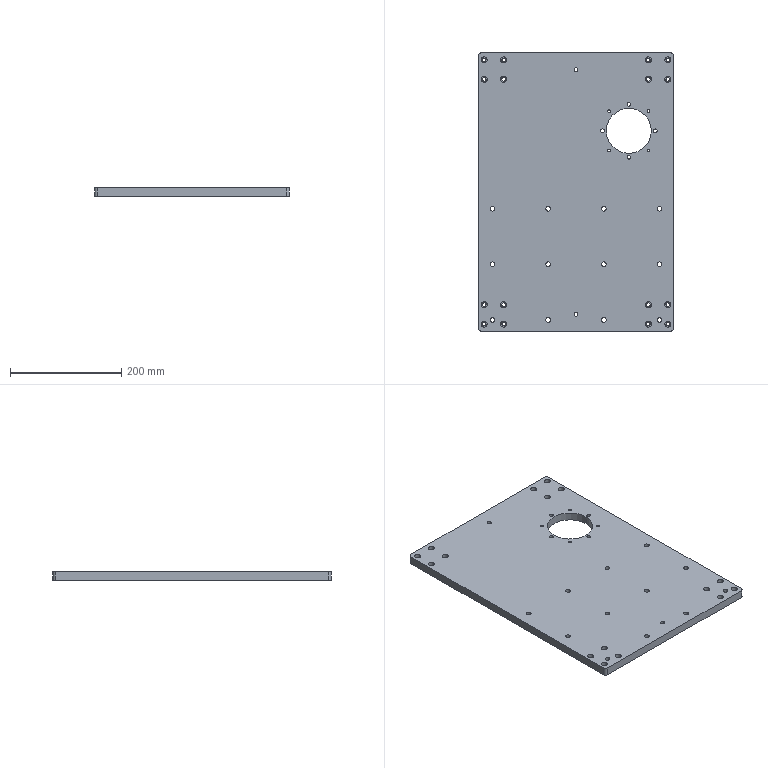NC program | Mastercam | posted with a generic post | part box 350 x 500 x 15 mm
Lines 3809 to 4195 of 4195:
N8380 T7 M6
N8390 G0 G90 G17 G54 X-245.4 Y176.45 A0. S7000 M3
N8400 G43 H7 Z50. M8
N8410 Z1.
N8420 G1 Z-.8 F600.
N8430 Y176.05 F1000.
N8440 G3 X-245. Y175.65 I.4 J0.
N8450 G1 X245.
N8460 G2 X250.65 Y170. I0. J-5.65
N8470 G1 Y-170.
N8480 G2 X245. Y-175.65 I-5.65 J0.
N8490 G1 X-245.
N8500 G2 X-250.65 Y-170. I0. J5.65
N8510 G1 Y170.
N8520 G2 X-245. Y175.65 I5.65 J0.
N8530 G3 X-244.6 Y176.05 I0. J.4
N8540 G1 Y176.45
N8550 G0 Z50.
N8560 X-237.1 Y169.05
N8570 Z1.
N8580 G1 Z-.8 F600.
N8590 Y169.45 F1000.
N8600 G3 X-237.5 Y169.85 I-.4 J0.
N8610 X-242.35 Y165. I0. J-4.85
N8620 X-237.5 Y160.15 I4.85 J0.
N8630 X-232.65 Y165. I0. J4.85
N8640 X-237.5 Y169.85 I-4.85 J0.
N8650 X-237.9 Y169.45 I0. J-.4
N8660 G1 Y169.05
N8670 G0 Z50.
N8680 X-202.1 Y134.05
N8690 Z1.
N8700 G1 Z-.8 F600.
N8710 Y134.45 F1000.
N8720 G3 X-202.5 Y134.85 I-.4 J0.
N8730 X-207.35 Y130. I0. J-4.85
N8740 X-202.5 Y125.15 I4.85 J0.
N8750 X-197.65 Y130. I0. J4.85
N8760 X-202.5 Y134.85 I-4.85 J0.
N8770 X-202.9 Y134.45 I0. J-.4
N8780 G1 Y134.05
N8790 G0 Z50.
N8800 X-202.1 Y169.05
N8810 Z1.
N8820 G1 Z-.8 F600.
N8830 Y169.45 F1000.
N8840 G3 X-202.5 Y169.85 I-.4 J0.
N8850 X-207.35 Y165. I0. J-4.85
N8860 X-202.5 Y160.15 I4.85 J0.
N8870 X-197.65 Y165. I0. J4.85
N8880 X-202.5 Y169.85 I-4.85 J0.
N8890 X-202.9 Y169.45 I0. J-.4
N8900 G1 Y169.05
N8910 G0 Z50.
N8920 X-237.1 Y134.05
N8930 Z1.
N8940 G1 Z-.8 F600.
N8950 Y134.45 F1000.
N8960 G3 X-237.5 Y134.85 I-.4 J0.
N8970 X-242.35 Y130. I0. J-4.85
N8980 X-237.5 Y125.15 I4.85 J0.
N8990 X-232.65 Y130. I0. J4.85
N9000 X-237.5 Y134.85 I-4.85 J0.
N9010 X-237.9 Y134.45 I0. J-.4
N9020 G1 Y134.05
N9030 G0 Z50.
N9040 X-237.1 Y-125.95
N9050 Z1.
N9060 G1 Z-.8 F600.
N9070 Y-125.55 F1000.
N9080 G3 X-237.5 Y-125.15 I-.4 J0.
N9090 X-242.35 Y-130. I0. J-4.85
N9100 X-237.5 Y-134.85 I4.85 J0.
N9110 X-232.65 Y-130. I0. J4.85
N9120 X-237.5 Y-125.15 I-4.85 J0.
N9130 X-237.9 Y-125.55 I0. J-.4
N9140 G1 Y-125.95
N9150 G0 Z50.
N9160 X-202.1 Y-160.95
N9170 Z1.
N9180 G1 Z-.8 F600.
N9190 Y-160.55 F1000.
N9200 G3 X-202.5 Y-160.15 I-.4 J0.
N9210 X-207.35 Y-165. I0. J-4.85
N9220 X-202.5 Y-169.85 I4.85 J0.
N9230 X-197.65 Y-165. I0. J4.85
N9240 X-202.5 Y-160.15 I-4.85 J0.
N9250 X-202.9 Y-160.55 I0. J-.4
N9260 G1 Y-160.95
N9270 G0 Z50.
N9280 X-202.1 Y-125.95
N9290 Z1.
N9300 G1 Z-.8 F600.
N9310 Y-125.55 F1000.
N9320 G3 X-202.5 Y-125.15 I-.4 J0.
N9330 X-207.35 Y-130. I0. J-4.85
N9340 X-202.5 Y-134.85 I4.85 J0.
N9350 X-197.65 Y-130. I0. J4.85
N9360 X-202.5 Y-125.15 I-4.85 J0.
N9370 X-202.9 Y-125.55 I0. J-.4
N9380 G1 Y-125.95
N9390 G0 Z50.
N9400 X-237.1 Y-160.95
N9410 Z1.
N9420 G1 Z-.8 F600.
N9430 Y-160.55 F1000.
N9440 G3 X-237.5 Y-160.15 I-.4 J0.
N9450 X-242.35 Y-165. I0. J-4.85
N9460 X-237.5 Y-169.85 I4.85 J0.
N9470 X-232.65 Y-165. I0. J4.85
N9480 X-237.5 Y-160.15 I-4.85 J0.
N9490 X-237.9 Y-160.55 I0. J-.4
N9500 G1 Y-160.95
N9510 G0 Z50.
N9520 X237.9 Y169.05
N9530 Z1.
N9540 G1 Z-.8 F600.
N9550 Y169.45 F1000.
N9560 G3 X237.5 Y169.85 I-.4 J0.
N9570 X232.65 Y165. I0. J-4.85
N9580 X237.5 Y160.15 I4.85 J0.
N9590 X242.35 Y165. I0. J4.85
N9600 X237.5 Y169.85 I-4.85 J0.
N9610 X237.1 Y169.45 I0. J-.4
N9620 G1 Y169.05
N9630 G0 Z50.
N9640 X202.9 Y134.05
N9650 Z1.
N9660 G1 Z-.8 F600.
N9670 Y134.45 F1000.
N9680 G3 X202.5 Y134.85 I-.4 J0.
N9690 X197.65 Y130. I0. J-4.85
N9700 X202.5 Y125.15 I4.85 J0.
N9710 X207.35 Y130. I0. J4.85
N9720 X202.5 Y134.85 I-4.85 J0.
N9730 X202.1 Y134.45 I0. J-.4
N9740 G1 Y134.05
N9750 G0 Z50.
N9760 X202.9 Y169.05
N9770 Z1.
N9780 G1 Z-.8 F600.
N9790 Y169.45 F1000.
N9800 G3 X202.5 Y169.85 I-.4 J0.
N9810 X197.65 Y165. I0. J-4.85
N9820 X202.5 Y160.15 I4.85 J0.
N9830 X207.35 Y165. I0. J4.85
N9840 X202.5 Y169.85 I-4.85 J0.
N9850 X202.1 Y169.45 I0. J-.4
N9860 G1 Y169.05
N9870 G0 Z50.
N9880 X237.9 Y134.05
N9890 Z1.
N9900 G1 Z-.8 F600.
N9910 Y134.45 F1000.
N9920 G3 X237.5 Y134.85 I-.4 J0.
N9930 X232.65 Y130. I0. J-4.85
N9940 X237.5 Y125.15 I4.85 J0.
N9950 X242.35 Y130. I0. J4.85
N9960 X237.5 Y134.85 I-4.85 J0.
N9970 X237.1 Y134.45 I0. J-.4
N9980 G1 Y134.05
N9990 G0 Z50.
N100 X237.9 Y-125.95
N110 Z1.
N120 G1 Z-.8 F600.
N130 Y-125.55 F1000.
N140 G3 X237.5 Y-125.15 I-.4 J0.
N150 X232.65 Y-130. I0. J-4.85
N160 X237.5 Y-134.85 I4.85 J0.
N170 X242.35 Y-130. I0. J4.85
N180 X237.5 Y-125.15 I-4.85 J0.
N190 X237.1 Y-125.55 I0. J-.4
N200 G1 Y-125.95
N210 G0 Z50.
N220 X202.9 Y-160.95
N230 Z1.
N240 G1 Z-.8 F600.
N250 Y-160.55 F1000.
N260 G3 X202.5 Y-160.15 I-.4 J0.
N270 X197.65 Y-165. I0. J-4.85
N280 X202.5 Y-169.85 I4.85 J0.
N290 X207.35 Y-165. I0. J4.85
N300 X202.5 Y-160.15 I-4.85 J0.
N310 X202.1 Y-160.55 I0. J-.4
N320 G1 Y-160.95
N330 G0 Z50.
N340 X202.9 Y-125.95
N350 Z1.
N360 G1 Z-.8 F600.
N370 Y-125.55 F1000.
N380 G3 X202.5 Y-125.15 I-.4 J0.
N390 X197.65 Y-130. I0. J-4.85
N400 X202.5 Y-134.85 I4.85 J0.
N410 X207.35 Y-130. I0. J4.85
N420 X202.5 Y-125.15 I-4.85 J0.
N430 X202.1 Y-125.55 I0. J-.4
N440 G1 Y-125.95
N450 G0 Z50.
N460 X237.9 Y-160.95
N470 Z1.
N480 G1 Z-.8 F600.
N490 Y-160.55 F1000.
N500 G3 X237.5 Y-160.15 I-.4 J0.
N510 X232.65 Y-165. I0. J-4.85
N520 X237.5 Y-169.85 I4.85 J0.
N530 X242.35 Y-165. I0. J4.85
N540 X237.5 Y-160.15 I-4.85 J0.
N550 X237.1 Y-160.55 I0. J-.4
N560 G1 Y-160.95
N570 G0 Z50.
N580 X-109.6 Y134.05
N590 Z1.
N600 G1 Z-.8 F600.
N610 Y134.45 F1000.
N620 G3 X-110. Y134.85 I-.4 J0.
N630 X-149.85 Y95. I0. J-39.85
N640 X-110. Y55.15 I39.85 J0.
N650 X-70.15 Y95. I0. J39.85
N660 X-110. Y134.85 I-39.85 J0.
N670 X-110.4 Y134.45 I0. J-.4
N680 G1 Y134.05
N690 G0 Z50.
N700 M5
N710 G91 G28 Z0. M9
N720 A0.
N730 M01
M00
( CL )
N740 T6 M6
N750 G0 G90 G17 G54 X-110. Y132.3 A0. S7000 M3
N760 G43 H6 Z50. M8
N770 Z1.
N780 G1 Z0. F600.
N790 G3 X-147.3 Y95. Z-.125 I0. J-37.3 F3000.
N800 X-110. Y57.7 Z-.25 I37.3 J0.
N810 X-72.7 Y95. Z-.375 I0. J37.3
N820 X-110. Y132.3 Z-.5 I-37.3 J0.
N830 X-147.3 Y95. Z-.625 I0. J-37.3
N840 X-110. Y57.7 Z-.75 I37.3 J0.
N850 X-72.7 Y95. Z-.875 I0. J37.3
N860 X-110. Y132.3 Z-1. I-37.3 J0.
N870 X-147.3 Y95. Z-1.125 I0. J-37.3
N880 X-110. Y57.7 Z-1.25 I37.3 J0.
N890 X-72.7 Y95. Z-1.375 I0. J37.3
N900 X-110. Y132.3 Z-1.5 I-37.3 J0.
N910 X-147.3 Y95. Z-1.625 I0. J-37.3
N920 X-110. Y57.7 Z-1.75 I37.3 J0.
N930 X-72.7 Y95. Z-1.875 I0. J37.3
N940 X-110. Y132.3 Z-2. I-37.3 J0.
N950 X-147.3 Y95. Z-2.125 I0. J-37.3
N960 X-110. Y57.7 Z-2.25 I37.3 J0.
N970 X-72.7 Y95. Z-2.375 I0. J37.3
N980 X-110. Y132.3 Z-2.5 I-37.3 J0.
N990 X-147.3 Y95. Z-2.625 I0. J-37.3
N1000 X-110. Y57.7 Z-2.75 I37.3 J0.
N1010 X-72.7 Y95. Z-2.875 I0. J37.3
N1020 X-110. Y132.3 Z-3. I-37.3 J0.
N1030 X-147.3 Y95. Z-3.125 I0. J-37.3
N1040 X-110. Y57.7 Z-3.25 I37.3 J0.
N1050 X-72.7 Y95. Z-3.375 I0. J37.3
N1060 X-110. Y132.3 Z-3.5 I-37.3 J0.
N1070 X-147.3 Y95. Z-3.625 I0. J-37.3
N1080 X-110. Y57.7 Z-3.75 I37.3 J0.
N1090 X-72.7 Y95. Z-3.875 I0. J37.3
N1100 X-110. Y132.3 Z-4. I-37.3 J0.
N1110 X-147.3 Y95. Z-4.125 I0. J-37.3
N1120 X-110. Y57.7 Z-4.25 I37.3 J0.
N1130 X-72.7 Y95. Z-4.375 I0. J37.3
N1140 X-110. Y132.3 Z-4.5 I-37.3 J0.
N1150 X-147.3 Y95. Z-4.625 I0. J-37.3
N1160 X-110. Y57.7 Z-4.75 I37.3 J0.
N1170 X-72.7 Y95. Z-4.875 I0. J37.3
N1180 X-110. Y132.3 Z-5. I-37.3 J0.
N1190 X-147.3 Y95. Z-5.125 I0. J-37.3
N1200 X-110. Y57.7 Z-5.25 I37.3 J0.
N1210 X-72.7 Y95. Z-5.375 I0. J37.3
N1220 X-110. Y132.3 Z-5.5 I-37.3 J0.
N1230 X-147.3 Y95. Z-5.625 I0. J-37.3
N1240 X-110. Y57.7 Z-5.75 I37.3 J0.
N1250 X-72.7 Y95. Z-5.875 I0. J37.3
N1260 X-110. Y132.3 Z-6. I-37.3 J0.
N1270 X-147.3 Y95. Z-6.125 I0. J-37.3
N1280 X-110. Y57.7 Z-6.25 I37.3 J0.
N1290 X-72.7 Y95. Z-6.375 I0. J37.3
N1300 X-110. Y132.3 Z-6.5 I-37.3 J0.
N1310 X-147.3 Y95. Z-6.625 I0. J-37.3
N1320 X-110. Y57.7 Z-6.75 I37.3 J0.
N1330 X-72.7 Y95. Z-6.875 I0. J37.3
N1340 X-110. Y132.3 Z-7. I-37.3 J0.
N1350 X-147.3 Y95. Z-7.125 I0. J-37.3
N1360 X-110. Y57.7 Z-7.25 I37.3 J0.
N1370 X-72.7 Y95. Z-7.375 I0. J37.3
N1380 X-110. Y132.3 Z-7.5 I-37.3 J0.
N1390 X-147.3 Y95. Z-7.625 I0. J-37.3
N1400 X-110. Y57.7 Z-7.75 I37.3 J0.
N1410 X-72.7 Y95. Z-7.875 I0. J37.3
N1420 X-110. Y132.3 Z-8. I-37.3 J0.
N1430 X-147.3 Y95. Z-8.125 I0. J-37.3
N1440 X-110. Y57.7 Z-8.25 I37.3 J0.
N1450 X-72.7 Y95. Z-8.375 I0. J37.3
N1460 X-110. Y132.3 Z-8.5 I-37.3 J0.
N1470 X-147.3 Y95. Z-8.625 I0. J-37.3
N1480 X-110. Y57.7 Z-8.75 I37.3 J0.
N1490 X-72.7 Y95. Z-8.875 I0. J37.3
N1500 X-110. Y132.3 Z-9. I-37.3 J0.
N1510 X-147.3 Y95. Z-9.125 I0. J-37.3
N1520 X-110. Y57.7 Z-9.25 I37.3 J0.
N1530 X-72.7 Y95. Z-9.375 I0. J37.3
N1540 X-110. Y132.3 Z-9.5 I-37.3 J0.
N1550 X-147.3 Y95. Z-9.625 I0. J-37.3
N1560 X-110. Y57.7 Z-9.75 I37.3 J0.
N1570 X-72.7 Y95. Z-9.875 I0. J37.3
N1580 X-110. Y132.3 Z-10. I-37.3 J0.
N1590 X-147.3 Y95. Z-10.125 I0. J-37.3
N1600 X-110. Y57.7 Z-10.25 I37.3 J0.
N1610 X-72.7 Y95. Z-10.375 I0. J37.3
N1620 X-110. Y132.3 Z-10.5 I-37.3 J0.
N1630 X-147.3 Y95. Z-10.625 I0. J-37.3
N1640 X-110. Y57.7 Z-10.75 I37.3 J0.
N1650 X-72.7 Y95. Z-10.875 I0. J37.3
N1660 X-110. Y132.3 Z-11. I-37.3 J0.
N1670 X-147.3 Y95. Z-11.125 I0. J-37.3
N1680 X-110. Y57.7 Z-11.25 I37.3 J0.
N1690 X-72.7 Y95. Z-11.375 I0. J37.3
N1700 X-110. Y132.3 Z-11.5 I-37.3 J0.
N1710 X-147.3 Y95. Z-11.625 I0. J-37.3
N1720 X-110. Y57.7 Z-11.75 I37.3 J0.
N1730 X-72.7 Y95. Z-11.875 I0. J37.3
N1740 X-110. Y132.3 Z-12. I-37.3 J0.
N1750 X-147.3 Y95. Z-12.125 I0. J-37.3
N1760 X-110. Y57.7 Z-12.25 I37.3 J0.
N1770 X-72.7 Y95. Z-12.375 I0. J37.3
N1780 X-110. Y132.3 Z-12.5 I-37.3 J0.
N1790 X-147.3 Y95. Z-12.625 I0. J-37.3
N1800 X-110. Y57.7 Z-12.75 I37.3 J0.
N1810 X-72.7 Y95. Z-12.875 I0. J37.3
N1820 X-110. Y132.3 Z-13. I-37.3 J0.
N1830 X-147.3 Y95. Z-13.125 I0. J-37.3
N1840 X-110. Y57.7 Z-13.25 I37.3 J0.
N1850 X-72.7 Y95. Z-13.375 I0. J37.3
N1860 X-110. Y132.3 Z-13.5 I-37.3 J0.
N1870 X-147.3 Y95. Z-13.625 I0. J-37.3
N1880 X-110. Y57.7 Z-13.75 I37.3 J0.
N1890 X-72.7 Y95. Z-13.875 I0. J37.3
N1900 X-110. Y132.3 Z-14. I-37.3 J0.
N1910 X-147.3 Y95. Z-14.125 I0. J-37.3
N1920 X-110. Y57.7 Z-14.25 I37.3 J0.
N1930 X-72.7 Y95. Z-14.375 I0. J37.3
N1940 X-110. Y132.3 Z-14.5 I-37.3 J0.
N1950 X-147.3 Y95. Z-14.625 I0. J-37.3
N1960 X-110. Y57.7 Z-14.75 I37.3 J0.
N1970 X-74.526 Y83.474 Z-14.85 I0. J37.3
N1980 X-72.7 Y95. I-35.474 J11.526
N1990 X-110. Y132.3 I-37.3 J0.
N2000 X-147.3 Y95. I0. J-37.3
N2010 X-110. Y57.7 I37.3 J0.
N2020 X-74.526 Y83.474 I0. J37.3
N2030 G0 Z50.
N2040 X-109.9 Y132.3
N2050 Z1.
N2060 G1 Z0. F600.
N2070 Y132.4 F1000.
N2080 G3 X-110. Y132.5 I-.1 J0.
N2090 X-147.5 Y95. Z-1.5 I0. J-37.5
N2100 X-110. Y57.5 Z-3. I37.5 J0.
N2110 X-72.5 Y95. Z-4.5 I0. J37.5
N2120 X-110. Y132.5 Z-6. I-37.5 J0.
N2130 X-147.5 Y95. Z-7.5 I0. J-37.5
N2140 X-110. Y57.5 Z-9. I37.5 J0.
N2150 X-72.5 Y95. Z-10.5 I0. J37.5
N2160 X-110. Y132.5 Z-12. I-37.5 J0.
N2170 X-147.5 Y95. Z-13.5 I0. J-37.5
N2180 X-115.866 Y57.962 Z-14.85 I37.5 J0.
N2190 X-110. Y57.5 I5.866 J37.038
N2200 X-72.5 Y95. I0. J37.5
N2210 X-110. Y132.5 I-37.5 J0.
N2220 X-147.5 Y95. I0. J-37.5
N2230 X-115.866 Y57.962 I37.5 J0.
N2240 X-115.851 Y57.961 I.015 J.098
N2250 X-115.752 Y58.045 I0. J.099
N2260 G1 X-115.736 Y58.144
N2270 G0 Z50.
N2280 M5
N2290 G91 G28 Z0. M9
N2300 G28 X0. Y0. A0.
N2310 M30
%